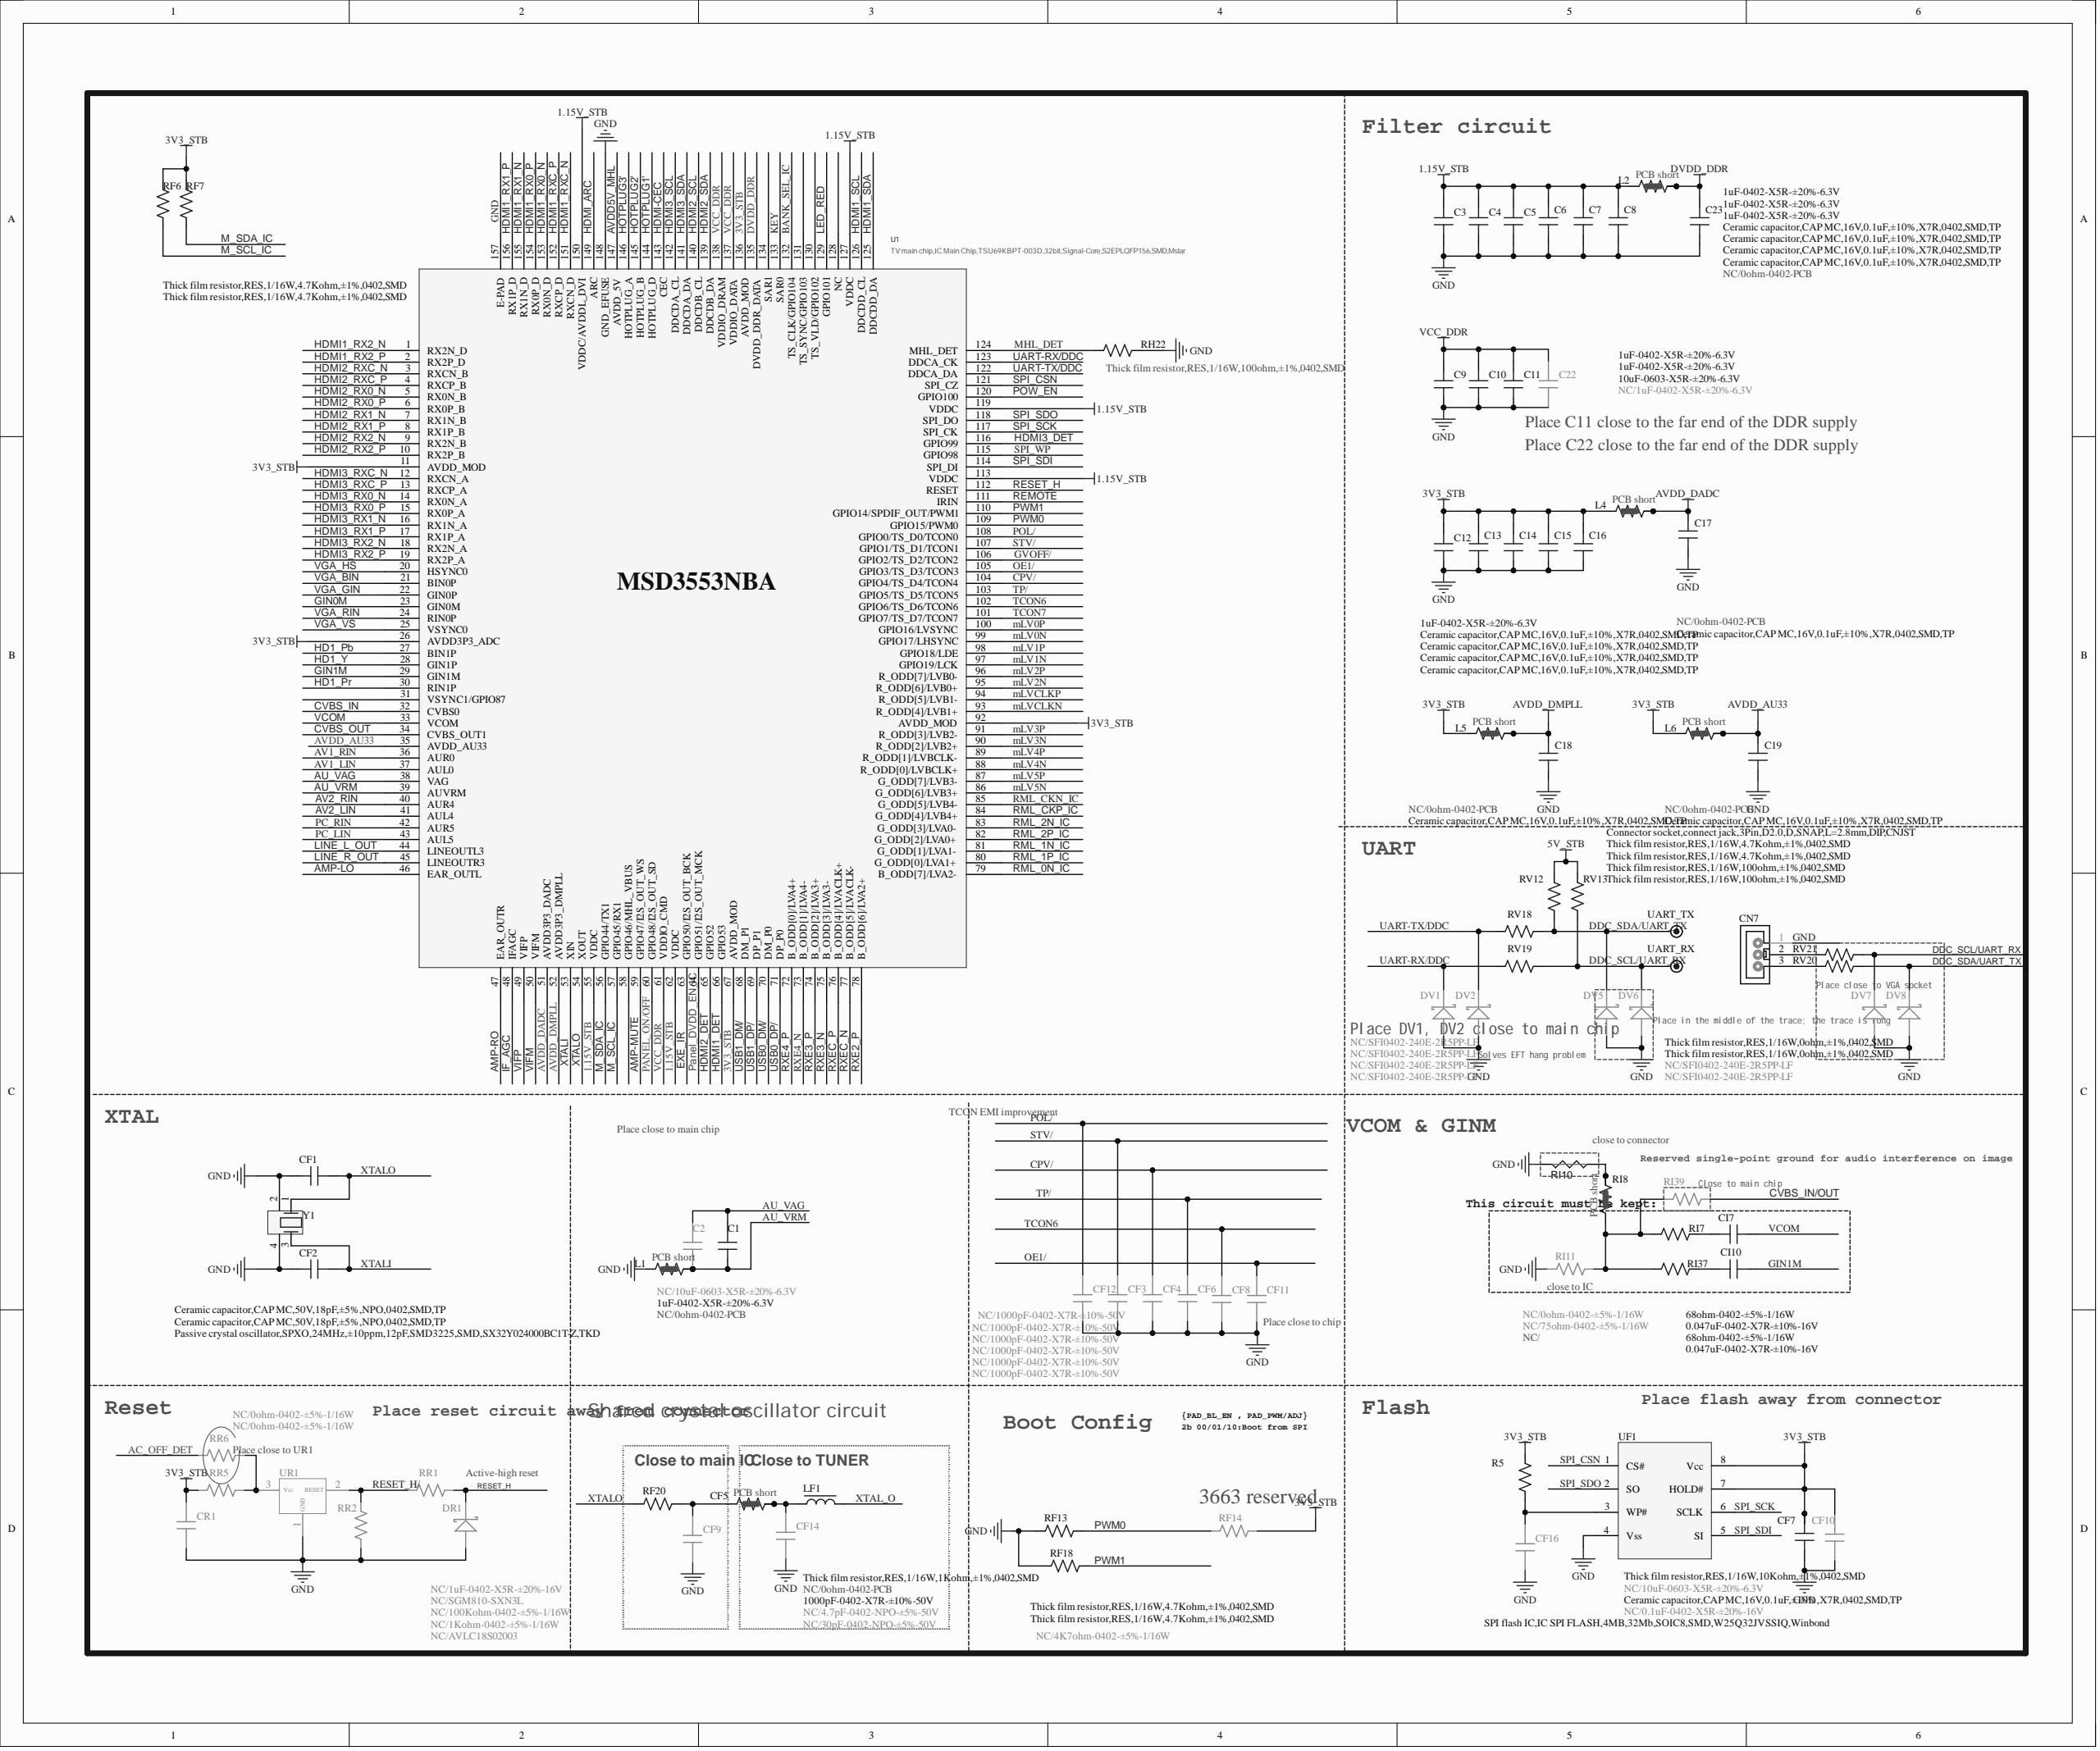Circuit board | Altium Designer | 719 parts | 352 nets | one sheet of the schematic
Parts on this sheet (reference | value | footprint):
C1 | 1uF-0402-X5R-±20%-6.3V | C0402
C2 | NC/10uF-0603-X5R-±20%-6.3V | C0603
C3 | 1uF-0402-X5R-±20%-6.3V | C0402
C4 | 1uF-0402-X5R-±20%-6.3V | C0402
C5 | 1uF-0402-X5R-±20%-6.3V | C0402
C6 | Ceramic capacitor,CAP MC,16V,0.1uF,±10%,X7R,0402,SMD,TP | C0402
C7 | Ceramic capacitor,CAP MC,16V,0.1uF,±10%,X7R,0402,SMD,TP | C0402
C8 | Ceramic capacitor,CAP MC,16V,0.1uF,±10%,X7R,0402,SMD,TP | C0402
C9 | 1uF-0402-X5R-±20%-6.3V | C0402
C10 | 1uF-0402-X5R-±20%-6.3V | C0402
C11 | 10uF-0603-X5R-±20%-6.3V | C0603
C12 | 1uF-0402-X5R-±20%-6.3V | C0402
C13 | Ceramic capacitor,CAP MC,16V,0.1uF,±10%,X7R,0402,SMD,TP | C0402
C14 | Ceramic capacitor,CAP MC,16V,0.1uF,±10%,X7R,0402,SMD,TP | C0402
C15 | Ceramic capacitor,CAP MC,16V,0.1uF,±10%,X7R,0402,SMD,TP | C0402
C16 | Ceramic capacitor,CAP MC,16V,0.1uF,±10%,X7R,0402,SMD,TP | C0402
C17 | Ceramic capacitor,CAP MC,16V,0.1uF,±10%,X7R,0402,SMD,TP | C0402
C18 | Ceramic capacitor,CAP MC,16V,0.1uF,±10%,X7R,0402,SMD,TP | C0402
C19 | Ceramic capacitor,CAP MC,16V,0.1uF,±10%,X7R,0402,SMD,TP | C0402
C22 | NC/1uF-0402-X5R-±20%-6.3V | C0402
C23 | Ceramic capacitor,CAP MC,16V,0.1uF,±10%,X7R,0402,SMD,TP | C0402
CF1 | Ceramic capacitor,CAP MC,50V,18pF,±5%,NPO,0402,SMD,TP | C0402
CF2 | Ceramic capacitor,CAP MC,50V,18pF,±5%,NPO,0402,SMD,TP | C0402
CF3 | NC/1000pF-0402-X7R-±10%-50V | C0402
CF4 | NC/1000pF-0402-X7R-±10%-50V | C0402
CF5 | NC/0ohm-0402-PCB | R0402SC
CF6 | NC/1000pF-0402-X7R-±10%-50V | C0402
CF7 | Ceramic capacitor,CAP MC,16V,0.1uF,±10%,X7R,0402,SMD,TP | C0402
CF8 | NC/1000pF-0402-X7R-±10%-50V | C0402
CF9 | NC/30pF-0402-NPO-±5%-50V | C0402
CF10 | NC/10uF-0603-X5R-±20%-6.3V | C0603
CF11 | NC/1000pF-0402-X7R-±10%-50V | C0402
CF12 | NC/1000pF-0402-X7R-±10%-50V | C0402
CF14 | NC/4.7pF-0402-NPO-±5%-50V | C0402
CF16 | NC/0.1uF-0402-X5R-±20%-16V | C0402
CI7 | 0.047uF-0402-X7R-±10%-16V | C0402
CI10 | 0.047uF-0402-X7R-±10%-16V | C0402
CN7 | Connector socket,connect jack,3Pin,D2.0,D,SNAP,L=2.8mm,DIP,CNJST | SIP3/2.0D-3
CR1 | NC/1uF-0402-X5R-±20%-16V | C0402
DR1 | NC/AVLC18S02003 | DIODE-S0402
DV1 | NC/SFI0402-240E-2R5PP-LF | DIODE-S0402
DV2 | NC/SFI0402-240E-2R5PP-LF | DIODE-S0402
DV5 | NC/SFI0402-240E-2R5PP-LF | DIODE-S0402
DV6 | NC/SFI0402-240E-2R5PP-LF | DIODE-S0402
DV7 | NC/SFI0402-240E-2R5PP-LF | DIODE-S0402
DV8 | NC/SFI0402-240E-2R5PP-LF | DIODE-S0402
L1 | NC/0ohm-0402-PCB | R0402SC
L2 | NC/0ohm-0402-PCB | R0402SC
L4 | NC/0ohm-0402-PCB | R0402SC
L5 | NC/0ohm-0402-PCB | R0402SC
L6 | NC/0ohm-0402-PCB | R0402SC
LF1 | 1000pF-0402-X7R-±10%-50V | L0402
R5 | Thick film resistor,RES,1/16W,10Kohm,±1%,0402,SMD | R0402
RF6 | Thick film resistor,RES,1/16W,4.7Kohm,±1%,0402,SMD | R0402
RF7 | Thick film resistor,RES,1/16W,4.7Kohm,±1%,0402,SMD | R0402
RF13 | Thick film resistor,RES,1/16W,4.7Kohm,±1%,0402,SMD | R0402
RF14 | NC/4K7ohm-0402-±5%-1/16W | R0402
RF18 | Thick film resistor,RES,1/16W,4.7Kohm,±1%,0402,SMD | R0402
RF20 | Thick film resistor,RES,1/16W,1Kohm,±1%,0402,SMD | R0402
RH22 | Thick film resistor,RES,1/16W,100ohm,±1%,0402,SMD | R0402
RI7 | 68ohm-0402-±5%-1/16W | R0402
RI8 | NC/ | R0402SC
RI10 | NC/SHORT | GND
RI11 | NC/0ohm-0402-±5%-1/16W | R0402
RI37 | 68ohm-0402-±5%-1/16W | R0402
RI39 | NC/75ohm-0402-±5%-1/16W | R0402
RR1 | NC/1Kohm-0402-±5%-1/16W | R0402
RR2 | NC/100Kohm-0402-±5%-1/16W | R0402
RR5 | NC/0ohm-0402-±5%-1/16W | R0402
RR6 | NC/0ohm-0402-±5%-1/16W | R0402
RV12 | Thick film resistor,RES,1/16W,4.7Kohm,±1%,0402,SMD | R0402
RV13 | Thick film resistor,RES,1/16W,4.7Kohm,±1%,0402,SMD | R0402
RV18 | Thick film resistor,RES,1/16W,100ohm,±1%,0402,SMD | R0402
RV19 | Thick film resistor,RES,1/16W,100ohm,±1%,0402,SMD | R0402
RV20 | Thick film resistor,RES,1/16W,0ohm,±1%,0402,SMD | R0402
RV21 | Thick film resistor,RES,1/16W,0ohm,±1%,0402,SMD | R0402
U1 | TV main chip,IC Main Chip,TSU69KBPT-003D,32bit,Signal-Core,S2EPLQFP156,SMD,Mstar | QFP156/0.4-2
UART_RX | TEST | TP
UART_TX | TEST | TP
UF1 | SPI flash IC,IC SPI FLASH,4MB,32Mb,SOIC8,SMD,W25Q32JVSSIQ,Winbond | SOIC8
UR1 | NC/SGM810-SXN3L | SO-23-1
Y1 | Passive crystal oscillator,SPXO,24MHz,±10ppm,12pF,SMD3225,SMD,SX32Y024000BC1T-Z,TKD | XTAL-S-3
Nets of these parts (net: part-pin ...):
XTALO: CF1-2 RF20-1 Y1-1 U1-54
XTALI: CF2-2 Y1-3 U1-53
XTAL_O: LF1-2
VIFP: U1-49
VIFM: U1-50
VGA_VS: U1-25
VGA_RIN: U1-24
VGA_HS: U1-20
VGA_GIN: U1-22
VGA_BIN: U1-21
VCOM: CI7-1 U1-33
VCC_DDR: C9-2 C10-2 C11-2 C22-2 U1-61 U1-137 U1-138
USB0_DP/: U1-71
USB0_DM/: U1-70
UART-TX/DDC: DV2-K RV18-1 U1-122
UART-RX/DDC: DV1-K RV19-1 U1-123
TP/: CF6-1 U1-103
TCON6: CF8-1 U1-102
STV/: CF3-1 U1-107
SPI_SDO: UF1-2 U1-118
SPI_SDI: UF1-5 U1-114
SPI_SCK: UF1-6 U1-117
SPI_CSN: UF1-1 U1-121
RESET_H/: RR1-2 RR2-1 UR1-2
RESET_H: DR1-K RR1-1 U1-112
REMOTE: U1-111
PWM1: RF18-1 U1-110
PWM0: RF13-1 RF14-2 U1-109
POW_EN: U1-120
POL/: CF12-1 U1-108
PANEL_ON/OFF: U1-60
Panel_DVDD_EN_IC: U1-64
OE1/: CF11-1 U1-105
NetRR5_1: RR5-1 RR6-1 UR1-3
NetRI8_2: RI8-2 RI8-3 RI10-JP_2K
NetRI7_2: RI7-2 RI8-1 RI11-2 RI37-2 RI39-2
NetCN7_3: CN7-3 RV20-1
NetCN7_2: CN7-2 RV21-1
NetCI10_2: CI10-2 RI37-1
NetCI7_2: CI7-2 RI7-1
NetCF16_1: CF16-1 R5-1 UF1-3
NetCF5_2: CF5-2 CF5-3 CF14-2 LF1-1
NetCF5_1: CF5-1 CF9-2 RF20-2
mLVCLKP: U1-94
mLVCLKN: U1-93
mLV5P: U1-87
mLV5N: U1-86
mLV4P: U1-89
mLV4N: U1-88
mLV3P: U1-91
mLV3N: U1-90
mLV2P: U1-96
mLV2N: U1-95
mLV1P: U1-98
mLV1N: U1-97
mLV0P: U1-100
mLV0N: U1-99
MHL_DET: RH22-2 U1-124
M_SDA_IC: RF7-1 U1-56
M_SCL_IC: RF6-1 U1-57
LINE_R_OUT: U1-45
LINE_L_OUT: U1-44
LED_RED: U1-129
KEY: U1-133
IF_AGC: U1-48
HOTPLUG2': U1-145
HDMI_ARC: U1-149
HDMI-CEC: U1-143
HDMI2_SDA: U1-139
HDMI2_SCL: U1-140
HDMI2_RXC_P: U1-4
HDMI2_RXC_N: U1-3
HDMI2_RX2_P: U1-10
HDMI2_RX2_N: U1-9
HDMI2_RX1_P: U1-8
HDMI2_RX1_N: U1-7
HDMI2_RX0_P: U1-6
HDMI2_RX0_N: U1-5
HDMI2_DET: U1-65
HD1_Y: U1-28
GVOFF/: U1-106
GND: C3-1 C4-1 C5-1 C6-1 C7-1 C8-1 C9-1 C10-1 C11-1 C12-1 C13-1 C14-1 C15-1 C16-1 C17-1 C18-1 C19-1 C22-1 C23-1 CF1-1 CF2-1 CF3-2 CF4-2 CF6-2 CF7-2 CF8-2 CF9-1 CF10-1 CF11-2 CF12-2 CF14-1 CF16-2 CN7-1 CR1-1 DR1-A DV1-A DV2-A DV5-A DV6-A DV7-A DV8-A L1-1 RF13-2 RF18-2 RH22-1 RI10-JP_1K RI11-1 RR2-2 UF1-4 UR1-1 Y1-2 Y1-4 U1-148 U1-157
GIN1M: CI10-1 U1-29
GIN0M: U1-23
EXE_IR: U1-63
DVDD_DDR: C23-2 L2-2 L2-3 U1-135
DDC_SDA/UART_TX: DV5-K DV8-K RV12-1 RV18-2 RV20-2 UART_TX-1
DDC_SCL/UART_RX: DV6-K DV7-K RV13-1 RV19-2 RV21-2 UART_RX-1
CVBS_OUT: U1-34
CVBS_IN/OUT: RI39-1
CVBS_IN: U1-32
CPV/: CF4-1 U1-104
AVDD_DMPLL: C18-2 L5-2 L5-3 U1-52
AVDD_DADC: C17-2 L4-2 L4-3 U1-51
AVDD_AU33: C19-2 L6-2 L6-3 U1-35
AV2_RIN: U1-40
AV2_LIN: U1-41
AV1_RIN: U1-36
AV1_LIN: U1-37
AU_VRM: C1-1 C2-1 L1-2 L1-3 U1-39
AU_VAG: C1-2 C2-2 U1-38
AMP-RO: U1-47
AMP-MUTE: U1-59
AMP-LO: U1-46
AC_OFF_DET: RR6-2
5V_STB: RV12-2 RV13-2
3V3_STB: C12-2 C13-2 C14-2 C15-2 C16-2 CF7-1 CF10-2 CR1-2 L4-1 L5-1 L6-1 R5-2 RF6-2 RF7-2 RF14-1 RR5-2 UF1-7 UF1-8 U1-11 U1-26 U1-67 U1-92 U1-136
1.15V_STB: C3-2 C4-2 C5-2 C6-2 C7-2 C8-2 L2-1 U1-55 U1-62 U1-113 U1-119 U1-127 U1-150